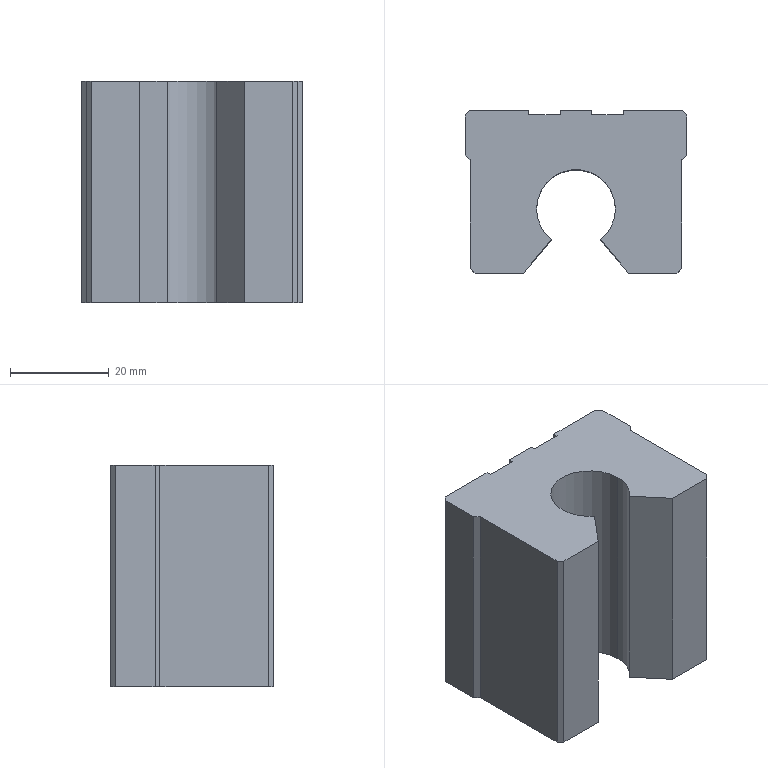Part | SolidWorks | features ICE 6, Chamfer 3, Draft 3, BaseBody 2, HoleWzd 2, Extrusion 1 | 1 solid | 52 faces | box 45 x 33 x 45 mm | volume 49974 mm3 | plane 25 | cone 16 | cylinder 11 | commonest cylinder face diameters 4.134 x8 16 x3
STEP:
#1=CARTESIAN_POINT('',(16.,44.567,212.933));
#2=VERTEX_POINT('',#1);
#3=CARTESIAN_POINT('',(16.,44.567,217.067));
#4=VERTEX_POINT('',#3);
#5=CARTESIAN_POINT('',(16.,44.567,215.));
#6=DIRECTION('',(0.,1.,0.));
#7=DIRECTION('',(0.,0.,-1.));
#8=AXIS2_PLACEMENT_3D('',#5,#6,#7);
#9=CIRCLE('',#8,2.067);
#10=EDGE_CURVE('',#2,#4,#9,.T.);
#11=ORIENTED_EDGE('',*,*,#10,.F.);
#12=CARTESIAN_POINT('',(16.,45.,212.5));
#13=VERTEX_POINT('',#12);
#14=CARTESIAN_POINT('',(16.,44.567,212.933));
#15=DIRECTION('',(0.,0.7071,-0.7071));
#16=VECTOR('',#15,1000.);
#17=LINE('',#14,#16);
#18=EDGE_CURVE('',#2,#13,#17,.T.);
#19=ORIENTED_EDGE('',*,*,#18,.T.);
#20=CARTESIAN_POINT('',(16.,45.,217.5));
#21=VERTEX_POINT('',#20);
#22=CARTESIAN_POINT('',(16.,45.,215.));
#23=DIRECTION('',(0.,-1.,0.));
#24=DIRECTION('',(0.,0.,-1.));
#25=AXIS2_PLACEMENT_3D('',#22,#23,#24);
#26=CIRCLE('',#25,2.5);
#27=EDGE_CURVE('',#21,#13,#26,.T.);
#28=ORIENTED_EDGE('',*,*,#27,.F.);
#29=CARTESIAN_POINT('',(16.,44.567,217.067));
#30=DIRECTION('',(0.,0.7071,0.7071));
#31=VECTOR('',#30,1000.);
#32=LINE('',#29,#31);
#33=EDGE_CURVE('',#4,#21,#32,.T.);
#34=ORIENTED_EDGE('',*,*,#33,.F.);
#35=EDGE_LOOP('',(#11,#19,#28,#34));
#36=FACE_OUTER_BOUND('',#35,.T.);
#37=CARTESIAN_POINT('',(16.,44.567,215.));
#38=DIRECTION('',(0.,1.,0.));
#39=DIRECTION('',(0.,0.,1.));
#40=AXIS2_PLACEMENT_3D('',#37,#38,#39);
#41=CONICAL_SURFACE('',#40,2.067,0.7854);
#42=ADVANCED_FACE('',(#36),#41,.F.);
#43=CARTESIAN_POINT('',(-16.,44.567,242.933));
#44=VERTEX_POINT('',#43);
#45=CARTESIAN_POINT('',(-16.,44.567,247.067));
#46=VERTEX_POINT('',#45);
#47=CARTESIAN_POINT('',(-16.,44.567,245.));
#48=DIRECTION('',(0.,1.,0.));
#49=DIRECTION('',(0.,0.,-1.));
#50=AXIS2_PLACEMENT_3D('',#47,#48,#49);
#51=CIRCLE('',#50,2.067);
#52=EDGE_CURVE('',#44,#46,#51,.T.);
#53=ORIENTED_EDGE('',*,*,#52,.F.);
#54=CARTESIAN_POINT('',(-16.,45.,242.5));
#55=VERTEX_POINT('',#54);
#56=CARTESIAN_POINT('',(-16.,44.567,242.933));
#57=DIRECTION('',(0.,0.7071,-0.7071));
#58=VECTOR('',#57,1000.);
#59=LINE('',#56,#58);
#60=EDGE_CURVE('',#44,#55,#59,.T.);
#61=ORIENTED_EDGE('',*,*,#60,.T.);
#62=CARTESIAN_POINT('',(-16.,45.,247.5));
#63=VERTEX_POINT('',#62);
#64=CARTESIAN_POINT('',(-16.,45.,245.));
#65=DIRECTION('',(0.,-1.,0.));
#66=DIRECTION('',(0.,0.,-1.));
#67=AXIS2_PLACEMENT_3D('',#64,#65,#66);
#68=CIRCLE('',#67,2.5);
#69=EDGE_CURVE('',#63,#55,#68,.T.);
#70=ORIENTED_EDGE('',*,*,#69,.F.);
#71=CARTESIAN_POINT('',(-16.,44.567,247.067));
#72=DIRECTION('',(0.,0.7071,0.7071));
#73=VECTOR('',#72,1000.);
#74=LINE('',#71,#73);
#75=EDGE_CURVE('',#46,#63,#74,.T.);
#76=ORIENTED_EDGE('',*,*,#75,.F.);
#77=EDGE_LOOP('',(#53,#61,#70,#76));
#78=FACE_OUTER_BOUND('',#77,.T.);
#79=CARTESIAN_POINT('',(-16.,44.567,245.));
#80=DIRECTION('',(0.,1.,0.));
#81=DIRECTION('',(0.,0.,1.));
#82=AXIS2_PLACEMENT_3D('',#79,#80,#81);
#83=CONICAL_SURFACE('',#82,2.067,0.7854);
#84=ADVANCED_FACE('',(#78),#83,.F.);
#85=CARTESIAN_POINT('',(16.,44.567,242.933));
#86=VERTEX_POINT('',#85);
#87=CARTESIAN_POINT('',(16.,44.567,247.067));
#88=VERTEX_POINT('',#87);
#89=CARTESIAN_POINT('',(16.,44.567,245.));
#90=DIRECTION('',(0.,1.,0.));
#91=DIRECTION('',(0.,0.,-1.));
#92=AXIS2_PLACEMENT_3D('',#89,#90,#91);
#93=CIRCLE('',#92,2.067);
#94=EDGE_CURVE('',#86,#88,#93,.T.);
#95=ORIENTED_EDGE('',*,*,#94,.F.);
#96=CARTESIAN_POINT('',(16.,45.,242.5));
#97=VERTEX_POINT('',#96);
#98=CARTESIAN_POINT('',(16.,44.567,242.933));
#99=DIRECTION('',(0.,0.7071,-0.7071));
#100=VECTOR('',#99,1000.);
#101=LINE('',#98,#100);
#102=EDGE_CURVE('',#86,#97,#101,.T.);
#103=ORIENTED_EDGE('',*,*,#102,.T.);
#104=CARTESIAN_POINT('',(16.,45.,247.5));
#105=VERTEX_POINT('',#104);
#106=CARTESIAN_POINT('',(16.,45.,245.));
#107=DIRECTION('',(0.,-1.,0.));
#108=DIRECTION('',(0.,0.,-1.));
#109=AXIS2_PLACEMENT_3D('',#106,#107,#108);
#110=CIRCLE('',#109,2.5);
#111=EDGE_CURVE('',#105,#97,#110,.T.);
#112=ORIENTED_EDGE('',*,*,#111,.F.);
#113=CARTESIAN_POINT('',(16.,44.567,247.067));
#114=DIRECTION('',(0.,0.7071,0.7071));
#115=VECTOR('',#114,1000.);
#116=LINE('',#113,#115);
#117=EDGE_CURVE('',#88,#105,#116,.T.);
#118=ORIENTED_EDGE('',*,*,#117,.F.);
#119=EDGE_LOOP('',(#95,#103,#112,#118));
#120=FACE_OUTER_BOUND('',#119,.T.);
#121=CARTESIAN_POINT('',(16.,44.567,245.));
#122=DIRECTION('',(0.,1.,0.));
#123=DIRECTION('',(0.,0.,1.));
#124=AXIS2_PLACEMENT_3D('',#121,#122,#123);
#125=CONICAL_SURFACE('',#124,2.067,0.7854);
#126=ADVANCED_FACE('',(#120),#125,.F.);
#127=CARTESIAN_POINT('',(-16.,44.567,212.933));
#128=VERTEX_POINT('',#127);
#129=CARTESIAN_POINT('',(-16.,44.567,217.067));
#130=VERTEX_POINT('',#129);
#131=CARTESIAN_POINT('',(-16.,44.567,215.));
#132=DIRECTION('',(0.,1.,0.));
#133=DIRECTION('',(0.,0.,-1.));
#134=AXIS2_PLACEMENT_3D('',#131,#132,#133);
#135=CIRCLE('',#134,2.067);
#136=EDGE_CURVE('',#128,#130,#135,.T.);
#137=ORIENTED_EDGE('',*,*,#136,.F.);
#138=CARTESIAN_POINT('',(-16.,45.,212.5));
#139=VERTEX_POINT('',#138);
#140=CARTESIAN_POINT('',(-16.,44.567,212.933));
#141=DIRECTION('',(0.,0.7071,-0.7071));
#142=VECTOR('',#141,1000.);
#143=LINE('',#140,#142);
#144=EDGE_CURVE('',#128,#139,#143,.T.);
#145=ORIENTED_EDGE('',*,*,#144,.T.);
#146=CARTESIAN_POINT('',(-16.,45.,217.5));
#147=VERTEX_POINT('',#146);
#148=CARTESIAN_POINT('',(-16.,45.,215.));
#149=DIRECTION('',(0.,-1.,0.));
#150=DIRECTION('',(0.,0.,-1.));
#151=AXIS2_PLACEMENT_3D('',#148,#149,#150);
#152=CIRCLE('',#151,2.5);
#153=EDGE_CURVE('',#147,#139,#152,.T.);
#154=ORIENTED_EDGE('',*,*,#153,.F.);
#155=CARTESIAN_POINT('',(-16.,44.567,217.067));
#156=DIRECTION('',(0.,0.7071,0.7071));
#157=VECTOR('',#156,1000.);
#158=LINE('',#155,#157);
#159=EDGE_CURVE('',#130,#147,#158,.T.);
#160=ORIENTED_EDGE('',*,*,#159,.F.);
#161=EDGE_LOOP('',(#137,#145,#154,#160));
#162=FACE_OUTER_BOUND('',#161,.T.);
#163=CARTESIAN_POINT('',(-16.,44.567,215.));
#164=DIRECTION('',(0.,1.,0.));
#165=DIRECTION('',(0.,0.,1.));
#166=AXIS2_PLACEMENT_3D('',#163,#164,#165);
#167=CONICAL_SURFACE('',#166,2.067,0.7854);
#168=ADVANCED_FACE('',(#162),#167,.F.);
#169=CARTESIAN_POINT('',(16.,29.393,212.933));
#170=VERTEX_POINT('',#169);
#171=CARTESIAN_POINT('',(16.,29.393,217.067));
#172=VERTEX_POINT('',#171);
#173=CARTESIAN_POINT('',(16.,29.393,215.));
#174=DIRECTION('',(0.,1.,0.));
#175=DIRECTION('',(0.,0.,1.));
#176=AXIS2_PLACEMENT_3D('',#173,#174,#175);
#177=CIRCLE('',#176,2.067);
#178=EDGE_CURVE('',#170,#172,#177,.T.);
#179=ORIENTED_EDGE('',*,*,#178,.F.);
#180=CARTESIAN_POINT('',(16.,45.,212.933));
#181=DIRECTION('',(0.,1.,0.));
#182=VECTOR('',#181,1000.);
#183=LINE('',#180,#182);
#184=EDGE_CURVE('',#170,#2,#183,.T.);
#185=ORIENTED_EDGE('',*,*,#184,.T.);
#186=ORIENTED_EDGE('',*,*,#10,.T.);
#187=CARTESIAN_POINT('',(16.,45.,217.067));
#188=DIRECTION('',(0.,1.,0.));
#189=VECTOR('',#188,1000.);
#190=LINE('',#187,#189);
#191=EDGE_CURVE('',#172,#4,#190,.T.);
#192=ORIENTED_EDGE('',*,*,#191,.F.);
#193=EDGE_LOOP('',(#179,#185,#186,#192));
#194=FACE_OUTER_BOUND('',#193,.T.);
#195=CARTESIAN_POINT('',(16.,45.,215.));
#196=DIRECTION('',(0.,1.,0.));
#197=DIRECTION('',(0.,0.,1.));
#198=AXIS2_PLACEMENT_3D('',#195,#196,#197);
#199=CYLINDRICAL_SURFACE('',#198,2.067);
#200=ADVANCED_FACE('',(#194),#199,.F.);
#201=CARTESIAN_POINT('',(16.,28.2,215.));
#202=VERTEX_POINT('',#201);
#203=CARTESIAN_POINT('',(16.,29.393,217.067));
#204=DIRECTION('',(0.,0.5,0.866));
#205=VECTOR('',#204,1000.);
#206=LINE('',#203,#205);
#207=EDGE_CURVE('',#202,#172,#206,.T.);
#208=ORIENTED_EDGE('',*,*,#207,.F.);
#209=CARTESIAN_POINT('',(16.,29.393,212.933));
#210=DIRECTION('',(0.,0.5,-0.866));
#211=VECTOR('',#210,1000.);
#212=LINE('',#209,#211);
#213=EDGE_CURVE('',#202,#170,#212,.T.);
#214=ORIENTED_EDGE('',*,*,#213,.T.);
#215=ORIENTED_EDGE('',*,*,#178,.T.);
#216=EDGE_LOOP('',(#208,#214,#215));
#217=FACE_OUTER_BOUND('',#216,.T.);
#218=CARTESIAN_POINT('',(16.,29.393,215.));
#219=DIRECTION('',(0.,1.,0.));
#220=DIRECTION('',(0.,0.,1.));
#221=AXIS2_PLACEMENT_3D('',#218,#219,#220);
#222=CONICAL_SURFACE('',#221,2.067,1.047);
#223=ADVANCED_FACE('',(#217),#222,.F.);
#224=CARTESIAN_POINT('',(16.,29.393,242.933));
#225=VERTEX_POINT('',#224);
#226=CARTESIAN_POINT('',(16.,29.393,247.067));
#227=VERTEX_POINT('',#226);
#228=CARTESIAN_POINT('',(16.,29.393,245.));
#229=DIRECTION('',(0.,1.,0.));
#230=DIRECTION('',(0.,0.,1.));
#231=AXIS2_PLACEMENT_3D('',#228,#229,#230);
#232=CIRCLE('',#231,2.067);
#233=EDGE_CURVE('',#225,#227,#232,.T.);
#234=ORIENTED_EDGE('',*,*,#233,.F.);
#235=CARTESIAN_POINT('',(16.,45.,242.933));
#236=DIRECTION('',(0.,1.,0.));
#237=VECTOR('',#236,1000.);
#238=LINE('',#235,#237);
#239=EDGE_CURVE('',#225,#86,#238,.T.);
#240=ORIENTED_EDGE('',*,*,#239,.T.);
#241=ORIENTED_EDGE('',*,*,#94,.T.);
#242=CARTESIAN_POINT('',(16.,45.,247.067));
#243=DIRECTION('',(0.,1.,0.));
#244=VECTOR('',#243,1000.);
#245=LINE('',#242,#244);
#246=EDGE_CURVE('',#227,#88,#245,.T.);
#247=ORIENTED_EDGE('',*,*,#246,.F.);
#248=EDGE_LOOP('',(#234,#240,#241,#247));
#249=FACE_OUTER_BOUND('',#248,.T.);
#250=CARTESIAN_POINT('',(16.,45.,245.));
#251=DIRECTION('',(0.,1.,0.));
#252=DIRECTION('',(0.,0.,1.));
#253=AXIS2_PLACEMENT_3D('',#250,#251,#252);
#254=CYLINDRICAL_SURFACE('',#253,2.067);
#255=ADVANCED_FACE('',(#249),#254,.F.);
#256=CARTESIAN_POINT('',(16.,28.2,245.));
#257=VERTEX_POINT('',#256);
#258=CARTESIAN_POINT('',(16.,29.393,247.067));
#259=DIRECTION('',(0.,0.5,0.866));
#260=VECTOR('',#259,1000.);
#261=LINE('',#258,#260);
#262=EDGE_CURVE('',#257,#227,#261,.T.);
#263=ORIENTED_EDGE('',*,*,#262,.F.);
#264=CARTESIAN_POINT('',(16.,29.393,242.933));
#265=DIRECTION('',(0.,0.5,-0.866));
#266=VECTOR('',#265,1000.);
#267=LINE('',#264,#266);
#268=EDGE_CURVE('',#257,#225,#267,.T.);
#269=ORIENTED_EDGE('',*,*,#268,.T.);
#270=ORIENTED_EDGE('',*,*,#233,.T.);
#271=EDGE_LOOP('',(#263,#269,#270));
#272=FACE_OUTER_BOUND('',#271,.T.);
#273=CARTESIAN_POINT('',(16.,29.393,245.));
#274=DIRECTION('',(0.,1.,0.));
#275=DIRECTION('',(0.,0.,1.));
#276=AXIS2_PLACEMENT_3D('',#273,#274,#275);
#277=CONICAL_SURFACE('',#276,2.067,1.047);
#278=ADVANCED_FACE('',(#272),#277,.F.);
#279=CARTESIAN_POINT('',(-16.,29.393,212.933));
#280=VERTEX_POINT('',#279);
#281=CARTESIAN_POINT('',(-16.,29.393,217.067));
#282=VERTEX_POINT('',#281);
#283=CARTESIAN_POINT('',(-16.,29.393,215.));
#284=DIRECTION('',(0.,1.,0.));
#285=DIRECTION('',(0.,0.,1.));
#286=AXIS2_PLACEMENT_3D('',#283,#284,#285);
#287=CIRCLE('',#286,2.067);
#288=EDGE_CURVE('',#280,#282,#287,.T.);
#289=ORIENTED_EDGE('',*,*,#288,.F.);
#290=CARTESIAN_POINT('',(-16.,45.,212.933));
#291=DIRECTION('',(0.,1.,0.));
#292=VECTOR('',#291,1000.);
#293=LINE('',#290,#292);
#294=EDGE_CURVE('',#280,#128,#293,.T.);
#295=ORIENTED_EDGE('',*,*,#294,.T.);
#296=ORIENTED_EDGE('',*,*,#136,.T.);
#297=CARTESIAN_POINT('',(-16.,45.,217.067));
#298=DIRECTION('',(0.,1.,0.));
#299=VECTOR('',#298,1000.);
#300=LINE('',#297,#299);
#301=EDGE_CURVE('',#282,#130,#300,.T.);
#302=ORIENTED_EDGE('',*,*,#301,.F.);
#303=EDGE_LOOP('',(#289,#295,#296,#302));
#304=FACE_OUTER_BOUND('',#303,.T.);
#305=CARTESIAN_POINT('',(-16.,45.,215.));
#306=DIRECTION('',(0.,1.,0.));
#307=DIRECTION('',(0.,0.,1.));
#308=AXIS2_PLACEMENT_3D('',#305,#306,#307);
#309=CYLINDRICAL_SURFACE('',#308,2.067);
#310=ADVANCED_FACE('',(#304),#309,.F.);
#311=CARTESIAN_POINT('',(-16.,28.2,215.));
#312=VERTEX_POINT('',#311);
#313=CARTESIAN_POINT('',(-16.,29.393,217.067));
#314=DIRECTION('',(0.,0.5,0.866));
#315=VECTOR('',#314,1000.);
#316=LINE('',#313,#315);
#317=EDGE_CURVE('',#312,#282,#316,.T.);
#318=ORIENTED_EDGE('',*,*,#317,.F.);
#319=CARTESIAN_POINT('',(-16.,29.393,212.933));
#320=DIRECTION('',(0.,0.5,-0.866));
#321=VECTOR('',#320,1000.);
#322=LINE('',#319,#321);
#323=EDGE_CURVE('',#312,#280,#322,.T.);
#324=ORIENTED_EDGE('',*,*,#323,.T.);
#325=ORIENTED_EDGE('',*,*,#288,.T.);
#326=EDGE_LOOP('',(#318,#324,#325));
#327=FACE_OUTER_BOUND('',#326,.T.);
#328=CARTESIAN_POINT('',(-16.,29.393,215.));
#329=DIRECTION('',(0.,1.,0.));
#330=DIRECTION('',(0.,0.,1.));
#331=AXIS2_PLACEMENT_3D('',#328,#329,#330);
#332=CONICAL_SURFACE('',#331,2.067,1.047);
#333=ADVANCED_FACE('',(#327),#332,.F.);
#334=CARTESIAN_POINT('',(-16.,29.393,242.933));
#335=VERTEX_POINT('',#334);
#336=CARTESIAN_POINT('',(-16.,29.393,247.067));
#337=VERTEX_POINT('',#336);
#338=CARTESIAN_POINT('',(-16.,29.393,245.));
#339=DIRECTION('',(0.,1.,0.));
#340=DIRECTION('',(0.,0.,1.));
#341=AXIS2_PLACEMENT_3D('',#338,#339,#340);
#342=CIRCLE('',#341,2.067);
#343=EDGE_CURVE('',#335,#337,#342,.T.);
#344=ORIENTED_EDGE('',*,*,#343,.F.);
#345=CARTESIAN_POINT('',(-16.,45.,242.933));
#346=DIRECTION('',(0.,1.,0.));
#347=VECTOR('',#346,1000.);
#348=LINE('',#345,#347);
#349=EDGE_CURVE('',#335,#44,#348,.T.);
#350=ORIENTED_EDGE('',*,*,#349,.T.);
#351=ORIENTED_EDGE('',*,*,#52,.T.);
#352=CARTESIAN_POINT('',(-16.,45.,247.067));
#353=DIRECTION('',(0.,1.,0.));
#354=VECTOR('',#353,1000.);
#355=LINE('',#352,#354);
#356=EDGE_CURVE('',#337,#46,#355,.T.);
#357=ORIENTED_EDGE('',*,*,#356,.F.);
#358=EDGE_LOOP('',(#344,#350,#351,#357));
#359=FACE_OUTER_BOUND('',#358,.T.);
#360=CARTESIAN_POINT('',(-16.,45.,245.));
#361=DIRECTION('',(0.,1.,0.));
#362=DIRECTION('',(0.,0.,1.));
#363=AXIS2_PLACEMENT_3D('',#360,#361,#362);
#364=CYLINDRICAL_SURFACE('',#363,2.067);
#365=ADVANCED_FACE('',(#359),#364,.F.);
#366=CARTESIAN_POINT('',(-16.,28.2,245.));
#367=VERTEX_POINT('',#366);
#368=CARTESIAN_POINT('',(-16.,29.393,247.067));
#369=DIRECTION('',(0.,0.5,0.866));
#370=VECTOR('',#369,1000.);
#371=LINE('',#368,#370);
#372=EDGE_CURVE('',#367,#337,#371,.T.);
#373=ORIENTED_EDGE('',*,*,#372,.F.);
#374=CARTESIAN_POINT('',(-16.,29.393,242.933));
#375=DIRECTION('',(0.,0.5,-0.866));
#376=VECTOR('',#375,1000.);
#377=LINE('',#374,#376);
#378=EDGE_CURVE('',#367,#335,#377,.T.);
#379=ORIENTED_EDGE('',*,*,#378,.T.);
#380=ORIENTED_EDGE('',*,*,#343,.T.);
#381=EDGE_LOOP('',(#373,#379,#380));
#382=FACE_OUTER_BOUND('',#381,.T.);
#383=CARTESIAN_POINT('',(-16.,29.393,245.));
#384=DIRECTION('',(0.,1.,0.));
#385=DIRECTION('',(0.,0.,1.));
#386=AXIS2_PLACEMENT_3D('',#383,#384,#385);
#387=CONICAL_SURFACE('',#386,2.067,1.047);
#388=ADVANCED_FACE('',(#382),#387,.F.);
#389=CARTESIAN_POINT('',(8.,25.,252.5));
#390=VERTEX_POINT('',#389);
#391=CARTESIAN_POINT('',(5.,18.755,252.5));
#392=VERTEX_POINT('',#391);
#393=CARTESIAN_POINT('',(0.,25.,252.5));
#394=DIRECTION('',(0.,0.,-1.));
#395=DIRECTION('',(-1.,0.,0.));
#396=AXIS2_PLACEMENT_3D('',#393,#394,#395);
#397=CIRCLE('',#396,8.);
#398=EDGE_CURVE('',#390,#392,#397,.T.);
#399=ORIENTED_EDGE('',*,*,#398,.F.);
#400=CARTESIAN_POINT('',(8.,25.,207.5));
#401=VERTEX_POINT('',#400);
#402=CARTESIAN_POINT('',(8.,25.,207.5));
#403=DIRECTION('',(0.,0.,-1.));
#404=VECTOR('',#403,1000.);
#405=LINE('',#402,#404);
#406=EDGE_CURVE('',#390,#401,#405,.T.);
#407=ORIENTED_EDGE('',*,*,#406,.T.);
#408=CARTESIAN_POINT('',(5.,18.755,207.5));
#409=VERTEX_POINT('',#408);
#410=CARTESIAN_POINT('',(0.,25.,207.5));
#411=DIRECTION('',(0.,0.,-1.));
#412=DIRECTION('',(-1.,0.,0.));
#413=AXIS2_PLACEMENT_3D('',#410,#411,#412);
#414=CIRCLE('',#413,8.);
#415=EDGE_CURVE('',#401,#409,#414,.T.);
#416=ORIENTED_EDGE('',*,*,#415,.T.);
#417=CARTESIAN_POINT('',(5.,18.755,207.5));
#418=DIRECTION('',(0.,0.,-1.));
#419=VECTOR('',#418,1000.);
#420=LINE('',#417,#419);
#421=EDGE_CURVE('',#392,#409,#420,.T.);
#422=ORIENTED_EDGE('',*,*,#421,.F.);
#423=EDGE_LOOP('',(#399,#407,#416,#422));
#424=FACE_OUTER_BOUND('',#423,.T.);
#425=CARTESIAN_POINT('',(0.,25.,207.5));
#426=DIRECTION('',(0.,0.,-1.));
#427=DIRECTION('',(-1.,0.,0.));
#428=AXIS2_PLACEMENT_3D('',#425,#426,#427);
#429=CYLINDRICAL_SURFACE('',#428,8.);
#430=ADVANCED_FACE('',(#424),#429,.F.);
#431=ORIENTED_EDGE('',*,*,#406,.F.);
#432=CARTESIAN_POINT('',(-8.,25.,252.5));
#433=VERTEX_POINT('',#432);
#434=CARTESIAN_POINT('',(0.,25.,252.5));
#435=DIRECTION('',(0.,0.,-1.));
#436=DIRECTION('',(-1.,0.,0.));
#437=AXIS2_PLACEMENT_3D('',#434,#435,#436);
#438=CIRCLE('',#437,8.);
#439=EDGE_CURVE('',#433,#390,#438,.T.);
#440=ORIENTED_EDGE('',*,*,#439,.F.);
#441=CARTESIAN_POINT('',(-8.,25.,207.5));
#442=VERTEX_POINT('',#441);
#443=CARTESIAN_POINT('',(-8.,25.,207.5));
#444=DIRECTION('',(0.,0.,-1.));
#445=VECTOR('',#444,1000.);
#446=LINE('',#443,#445);
#447=EDGE_CURVE('',#433,#442,#446,.T.);
#448=ORIENTED_EDGE('',*,*,#447,.T.);
#449=CARTESIAN_POINT('',(0.,25.,207.5));
#450=DIRECTION('',(0.,0.,-1.));
#451=DIRECTION('',(-1.,0.,0.));
#452=AXIS2_PLACEMENT_3D('',#449,#450,#451);
#453=CIRCLE('',#452,8.);
#454=EDGE_CURVE('',#442,#401,#453,.T.);
#455=ORIENTED_EDGE('',*,*,#454,.T.);
#456=EDGE_LOOP('',(#431,#440,#448,#455));
#457=FACE_OUTER_BOUND('',#456,.T.);
#458=CARTESIAN_POINT('',(0.,25.,207.5));
#459=DIRECTION('',(0.,0.,-1.));
#460=DIRECTION('',(-1.,0.,0.));
#461=AXIS2_PLACEMENT_3D('',#458,#459,#460);
#462=CYLINDRICAL_SURFACE('',#461,8.);
#463=ADVANCED_FACE('',(#457),#462,.F.);
#464=CARTESIAN_POINT('',(-9.6,45.,252.5));
#465=VERTEX_POINT('',#464);
#466=CARTESIAN_POINT('',(-21.6,45.,252.5));
#467=VERTEX_POINT('',#466);
#468=CARTESIAN_POINT('',(22.5,45.,252.5));
#469=DIRECTION('',(-1.,0.,0.));
#470=VECTOR('',#469,1000.);
#471=LINE('',#468,#470);
#472=EDGE_CURVE('',#465,#467,#471,.T.);
#473=ORIENTED_EDGE('',*,*,#472,.T.);
#474=CARTESIAN_POINT('',(-22.5,44.1,252.5));
#475=VERTEX_POINT('',#474);
#476=CARTESIAN_POINT('',(0.45,67.05,252.5));
#477=DIRECTION('',(-0.7071,-0.7071,0.));
#478=VECTOR('',#477,1000.);
#479=LINE('',#476,#478);
#480=EDGE_CURVE('',#467,#475,#479,.T.);
#481=ORIENTED_EDGE('',*,*,#480,.T.);
#482=CARTESIAN_POINT('',(-22.5,36.,252.5));
#483=VERTEX_POINT('',#482);
#484=CARTESIAN_POINT('',(-22.5,45.,252.5));
#485=DIRECTION('',(0.,-1.,0.));
#486=VECTOR('',#485,1000.);
#487=LINE('',#484,#486);
#488=EDGE_CURVE('',#475,#483,#487,.T.);
#489=ORIENTED_EDGE('',*,*,#488,.T.);
#490=CARTESIAN_POINT('',(-21.5,35.,252.5));
#491=VERTEX_POINT('',#490);
#492=CARTESIAN_POINT('',(-4.5,18.,252.5));
#493=DIRECTION('',(-0.7071,0.7071,0.));
#494=VECTOR('',#493,1000.);
#495=LINE('',#492,#494);
#496=EDGE_CURVE('',#491,#483,#495,.T.);
#497=ORIENTED_EDGE('',*,*,#496,.F.);
#498=CARTESIAN_POINT('',(-21.5,13.,252.5));
#499=VERTEX_POINT('',#498);
#500=CARTESIAN_POINT('',(-21.5,12.,252.5));
#501=DIRECTION('',(0.,1.,0.));
#502=VECTOR('',#501,1000.);
#503=LINE('',#500,#502);
#504=EDGE_CURVE('',#499,#491,#503,.T.);
#505=ORIENTED_EDGE('',*,*,#504,.F.);
#506=CARTESIAN_POINT('',(-20.5,12.,252.5));
#507=VERTEX_POINT('',#506);
#508=CARTESIAN_POINT('',(-15.5,7.,252.5));
#509=DIRECTION('',(0.7071,-0.7071,0.));
#510=VECTOR('',#509,1000.);
#511=LINE('',#508,#510);
#512=EDGE_CURVE('',#499,#507,#511,.T.);
#513=ORIENTED_EDGE('',*,*,#512,.T.);
#514=CARTESIAN_POINT('',(-10.668,12.,252.5));
#515=VERTEX_POINT('',#514);
#516=CARTESIAN_POINT('',(22.5,12.,252.5));
#517=DIRECTION('',(-1.,0.,0.));
#518=VECTOR('',#517,1000.);
#519=LINE('',#516,#518);
#520=EDGE_CURVE('',#515,#507,#519,.T.);
#521=ORIENTED_EDGE('',*,*,#520,.F.);
#522=CARTESIAN_POINT('',(-5.,18.755,252.5));
#523=VERTEX_POINT('',#522);
#524=CARTESIAN_POINT('',(19.285,47.697,252.5));
#525=DIRECTION('',(-0.6428,-0.766,0.));
#526=VECTOR('',#525,1000.);
#527=LINE('',#524,#526);
#528=EDGE_CURVE('',#523,#515,#527,.T.);
#529=ORIENTED_EDGE('',*,*,#528,.F.);
#530=CARTESIAN_POINT('',(0.,25.,252.5));
#531=DIRECTION('',(0.,0.,-1.));
#532=DIRECTION('',(-1.,0.,0.));
#533=AXIS2_PLACEMENT_3D('',#530,#531,#532);
#534=CIRCLE('',#533,8.);
#535=EDGE_CURVE('',#523,#433,#534,.T.);
#536=ORIENTED_EDGE('',*,*,#535,.T.);
#537=ORIENTED_EDGE('',*,*,#439,.T.);
#538=ORIENTED_EDGE('',*,*,#398,.T.);
#539=CARTESIAN_POINT('',(10.668,12.,252.5));
#540=VERTEX_POINT('',#539);
#541=CARTESIAN_POINT('',(10.668,12.,252.5));
#542=CARTESIAN_POINT('',(8.779,14.252,252.5));
#543=CARTESIAN_POINT('',(6.889,16.503,252.5));
#544=CARTESIAN_POINT('',(5.,18.755,252.5));
#545=B_SPLINE_CURVE_WITH_KNOTS('',3,(#541,#542,#543,#544),.UNSPECIFIED.,.F.,.F.,(4,4),(0.,1.),.UNSPECIFIED.);
#546=EDGE_CURVE('',#540,#392,#545,.T.);
#547=ORIENTED_EDGE('',*,*,#546,.F.);
#548=CARTESIAN_POINT('',(20.5,12.,252.5));
#549=VERTEX_POINT('',#548);
#550=CARTESIAN_POINT('',(22.5,12.,252.5));
#551=DIRECTION('',(-1.,0.,0.));
#552=VECTOR('',#551,1000.);
#553=LINE('',#550,#552);
#554=EDGE_CURVE('',#549,#540,#553,.T.);
#555=ORIENTED_EDGE('',*,*,#554,.F.);
#556=CARTESIAN_POINT('',(21.5,13.,252.5));
#557=VERTEX_POINT('',#556);
#558=CARTESIAN_POINT('',(38.,29.5,252.5));
#559=DIRECTION('',(0.7071,0.7071,0.));
#560=VECTOR('',#559,1000.);
#561=LINE('',#558,#560);
#562=EDGE_CURVE('',#549,#557,#561,.T.);
#563=ORIENTED_EDGE('',*,*,#562,.T.);
#564=CARTESIAN_POINT('',(21.5,35.,252.5));
#565=VERTEX_POINT('',#564);
#566=CARTESIAN_POINT('',(21.5,36.,252.5));
#567=DIRECTION('',(0.,-1.,0.));
#568=VECTOR('',#567,1000.);
#569=LINE('',#566,#568);
#570=EDGE_CURVE('',#565,#557,#569,.T.);
#571=ORIENTED_EDGE('',*,*,#570,.F.);
#572=CARTESIAN_POINT('',(22.5,36.,252.5));
#573=VERTEX_POINT('',#572);
#574=CARTESIAN_POINT('',(27.,40.5,252.5));
#575=DIRECTION('',(-0.7071,-0.7071,0.));
#576=VECTOR('',#575,1000.);
#577=LINE('',#574,#576);
#578=EDGE_CURVE('',#573,#565,#577,.T.);
#579=ORIENTED_EDGE('',*,*,#578,.F.);
#580=CARTESIAN_POINT('',(22.5,44.1,252.5));
#581=VERTEX_POINT('',#580);
#582=CARTESIAN_POINT('',(22.5,45.,252.5));
#583=DIRECTION('',(0.,-1.,0.));
#584=VECTOR('',#583,1000.);
#585=LINE('',#582,#584);
#586=EDGE_CURVE('',#581,#573,#585,.T.);
#587=ORIENTED_EDGE('',*,*,#586,.F.);
#588=CARTESIAN_POINT('',(21.6,45.,252.5));
#589=VERTEX_POINT('',#588);
#590=CARTESIAN_POINT('',(22.05,44.55,252.5));
#591=DIRECTION('',(-0.7071,0.7071,0.));
#592=VECTOR('',#591,1000.);
#593=LINE('',#590,#592);
#594=EDGE_CURVE('',#581,#589,#593,.T.);
#595=ORIENTED_EDGE('',*,*,#594,.T.);
#596=CARTESIAN_POINT('',(9.6,45.,252.5));
#597=VERTEX_POINT('',#596);
#598=CARTESIAN_POINT('',(22.5,45.,252.5));
#599=DIRECTION('',(-1.,0.,0.));
#600=VECTOR('',#599,1000.);
#601=LINE('',#598,#600);
#602=EDGE_CURVE('',#589,#597,#601,.T.);
#603=ORIENTED_EDGE('',*,*,#602,.T.);
#604=CARTESIAN_POINT('',(9.6,44.1,252.5));
#605=VERTEX_POINT('',#604);
#606=CARTESIAN_POINT('',(9.6,44.1,252.5));
#607=DIRECTION('',(0.,1.,0.));
#608=VECTOR('',#607,1000.);
#609=LINE('',#606,#608);
#610=EDGE_CURVE('',#605,#597,#609,.T.);
#611=ORIENTED_EDGE('',*,*,#610,.F.);
#612=CARTESIAN_POINT('',(3.2,44.1,252.5));
#613=VERTEX_POINT('',#612);
#614=CARTESIAN_POINT('',(3.2,44.1,252.5));
#615=DIRECTION('',(1.,0.,0.));
#616=VECTOR('',#615,1000.);
#617=LINE('',#614,#616);
#618=EDGE_CURVE('',#613,#605,#617,.T.);
#619=ORIENTED_EDGE('',*,*,#618,.F.);
#620=CARTESIAN_POINT('',(3.2,45.,252.5));
#621=VERTEX_POINT('',#620);
#622=CARTESIAN_POINT('',(3.2,45.,252.5));
#623=DIRECTION('',(0.,-1.,0.));
#624=VECTOR('',#623,1000.);
#625=LINE('',#622,#624);
#626=EDGE_CURVE('',#621,#613,#625,.T.);
#627=ORIENTED_EDGE('',*,*,#626,.F.);
#628=CARTESIAN_POINT('',(-3.2,45.,252.5));
#629=VERTEX_POINT('',#628);
#630=CARTESIAN_POINT('',(22.5,45.,252.5));
#631=DIRECTION('',(-1.,0.,0.));
#632=VECTOR('',#631,1000.);
#633=LINE('',#630,#632);
#634=EDGE_CURVE('',#621,#629,#633,.T.);
#635=ORIENTED_EDGE('',*,*,#634,.T.);
#636=CARTESIAN_POINT('',(-3.2,44.1,252.5));
#637=VERTEX_POINT('',#636);
#638=CARTESIAN_POINT('',(-3.2,44.1,252.5));
#639=DIRECTION('',(0.,1.,0.));
#640=VECTOR('',#639,1000.);
#641=LINE('',#638,#640);
#642=EDGE_CURVE('',#637,#629,#641,.T.);
#643=ORIENTED_EDGE('',*,*,#642,.F.);
#644=CARTESIAN_POINT('',(-9.6,44.1,252.5));
#645=VERTEX_POINT('',#644);
#646=CARTESIAN_POINT('',(-9.6,44.1,252.5));
#647=DIRECTION('',(1.,0.,0.));
#648=VECTOR('',#647,1000.);
#649=LINE('',#646,#648);
#650=EDGE_CURVE('',#645,#637,#649,.T.);
#651=ORIENTED_EDGE('',*,*,#650,.F.);
#652=CARTESIAN_POINT('',(-9.6,45.,252.5));
#653=DIRECTION('',(0.,-1.,0.));
#654=VECTOR('',#653,1000.);
#655=LINE('',#652,#654);
#656=EDGE_CURVE('',#465,#645,#655,.T.);
#657=ORIENTED_EDGE('',*,*,#656,.F.);
#658=EDGE_LOOP('',(#473,#481,#489,#497,#505,#513,#521,#529,#536,#537,#538,#547,#555,#563,#571,#579,#587,#595,#603,#611,#619,#627,#635,#643,#651,#657));
#659=FACE_OUTER_BOUND('',#658,.T.);
#660=CARTESIAN_POINT('',(22.5,45.,252.5));
#661=DIRECTION('',(0.,0.,1.));
#662=DIRECTION('',(1.,0.,0.));
#663=AXIS2_PLACEMENT_3D('',#660,#661,#662);
#664=PLANE('',#663);
#665=ADVANCED_FACE('',(#659),#664,.T.);
#666=ORIENTED_EDGE('',*,*,#520,.T.);
#667=CARTESIAN_POINT('',(-20.5,12.,207.5));
#668=VERTEX_POINT('',#667);
#669=CARTESIAN_POINT('',(-20.5,12.,207.5));
#670=DIRECTION('',(0.,0.,-1.));
#671=VECTOR('',#670,1000.);
#672=LINE('',#669,#671);
#673=EDGE_CURVE('',#507,#668,#672,.T.);
#674=ORIENTED_EDGE('',*,*,#673,.T.);
#675=CARTESIAN_POINT('',(-10.668,12.,207.5));
#676=VERTEX_POINT('',#675);
#677=CARTESIAN_POINT('',(-22.5,12.,207.5));
#678=DIRECTION('',(1.,0.,0.));
#679=VECTOR('',#678,1000.);
#680=LINE('',#677,#679);
#681=EDGE_CURVE('',#668,#676,#680,.T.);
#682=ORIENTED_EDGE('',*,*,#681,.T.);
#683=CARTESIAN_POINT('',(-10.668,12.,207.5));
#684=DIRECTION('',(0.,0.,1.));
#685=VECTOR('',#684,1000.);
#686=LINE('',#683,#685);
#687=EDGE_CURVE('',#676,#515,#686,.T.);
#688=ORIENTED_EDGE('',*,*,#687,.T.);
#689=EDGE_LOOP('',(#666,#674,#682,#688));
#690=FACE_OUTER_BOUND('',#689,.T.);
#691=CARTESIAN_POINT('',(0.,12.,0.));
#692=DIRECTION('',(0.,-1.,0.));
#693=DIRECTION('',(0.,0.,-1.));
#694=AXIS2_PLACEMENT_3D('',#691,#692,#693);
#695=PLANE('',#694);
#696=ADVANCED_FACE('',(#690),#695,.T.);
#697=ORIENTED_EDGE('',*,*,#111,.T.);
#698=CARTESIAN_POINT('',(16.,45.,245.));
#699=DIRECTION('',(0.,-1.,0.));
#700=DIRECTION('',(0.,0.,-1.));
#701=AXIS2_PLACEMENT_3D('',#698,#699,#700);
#702=CIRCLE('',#701,2.5);
#703=EDGE_CURVE('',#97,#105,#702,.T.);
#704=ORIENTED_EDGE('',*,*,#703,.T.);
#705=EDGE_LOOP('',(#697,#704));
#706=FACE_BOUND('',#705,.T.);
#707=ORIENTED_EDGE('',*,*,#27,.T.);
#708=CARTESIAN_POINT('',(16.,45.,215.));
#709=DIRECTION('',(0.,-1.,0.));
#710=DIRECTION('',(0.,0.,-1.));
#711=AXIS2_PLACEMENT_3D('',#708,#709,#710);
#712=CIRCLE('',#711,2.5);
#713=EDGE_CURVE('',#13,#21,#712,.T.);
#714=ORIENTED_EDGE('',*,*,#713,.T.);
#715=EDGE_LOOP('',(#707,#714));
#716=FACE_BOUND('',#715,.T.);
#717=ORIENTED_EDGE('',*,*,#602,.F.);
#718=CARTESIAN_POINT('',(21.6,45.,207.5));
#719=VERTEX_POINT('',#718);
#720=CARTESIAN_POINT('',(21.6,45.,207.5));
#721=DIRECTION('',(0.,0.,-1.));
#722=VECTOR('',#721,1000.);
#723=LINE('',#720,#722);
#724=EDGE_CURVE('',#589,#719,#723,.T.);
#725=ORIENTED_EDGE('',*,*,#724,.T.);
#726=CARTESIAN_POINT('',(9.6,45.,207.5));
#727=VERTEX_POINT('',#726);
#728=CARTESIAN_POINT('',(-22.5,45.,207.5));
#729=DIRECTION('',(1.,0.,0.));
#730=VECTOR('',#729,1000.);
#731=LINE('',#728,#730);
#732=EDGE_CURVE('',#727,#719,#731,.T.);
#733=ORIENTED_EDGE('',*,*,#732,.F.);
#734=CARTESIAN_POINT('',(9.6,45.,207.5));
#735=DIRECTION('',(0.,0.,1.));
#736=VECTOR('',#735,1000.);
#737=LINE('',#734,#736);
#738=EDGE_CURVE('',#727,#597,#737,.T.);
#739=ORIENTED_EDGE('',*,*,#738,.T.);
#740=EDGE_LOOP('',(#717,#725,#733,#739));
#741=FACE_OUTER_BOUND('',#740,.T.);
#742=CARTESIAN_POINT('',(0.,45.,0.));
#743=DIRECTION('',(0.,-1.,0.));
#744=DIRECTION('',(0.,0.,-1.));
#745=AXIS2_PLACEMENT_3D('',#742,#743,#744);
#746=PLANE('',#745);
#747=ADVANCED_FACE('',(#706,#716,#741),#746,.F.);
#748=ORIENTED_EDGE('',*,*,#634,.F.);
#749=CARTESIAN_POINT('',(3.2,45.,207.5));
#750=VERTEX_POINT('',#749);
#751=CARTESIAN_POINT('',(3.2,45.,207.5));
#752=DIRECTION('',(0.,0.,1.));
#753=VECTOR('',#752,1000.);
#754=LINE('',#751,#753);
#755=EDGE_CURVE('',#750,#621,#754,.T.);
#756=ORIENTED_EDGE('',*,*,#755,.F.);
#757=CARTESIAN_POINT('',(-3.2,45.,207.5));
#758=VERTEX_POINT('',#757);
#759=CARTESIAN_POINT('',(-22.5,45.,207.5));
#760=DIRECTION('',(1.,0.,0.));
#761=VECTOR('',#760,1000.);
#762=LINE('',#759,#761);
#763=EDGE_CURVE('',#758,#750,#762,.T.);
#764=ORIENTED_EDGE('',*,*,#763,.F.);
#765=CARTESIAN_POINT('',(-3.2,45.,207.5));
#766=DIRECTION('',(0.,0.,1.));
#767=VECTOR('',#766,1000.);
#768=LINE('',#765,#767);
#769=EDGE_CURVE('',#758,#629,#768,.T.);
#770=ORIENTED_EDGE('',*,*,#769,.T.);
#771=EDGE_LOOP('',(#748,#756,#764,#770));
#772=FACE_OUTER_BOUND('',#771,.T.);
#773=CARTESIAN_POINT('',(0.,45.,0.));
#774=DIRECTION('',(0.,-1.,0.));
#775=DIRECTION('',(0.,0.,-1.));
#776=AXIS2_PLACEMENT_3D('',#773,#774,#775);
#777=PLANE('',#776);
#778=ADVANCED_FACE('',(#772),#777,.F.);
#779=CARTESIAN_POINT('',(22.5,44.1,207.5));
#780=VERTEX_POINT('',#779);
#781=CARTESIAN_POINT('',(22.5,36.,207.5));
#782=VERTEX_POINT('',#781);
#783=CARTESIAN_POINT('',(22.5,45.,207.5));
#784=DIRECTION('',(0.,-1.,0.));
#785=VECTOR('',#784,1000.);
#786=LINE('',#783,#785);
#787=EDGE_CURVE('',#780,#782,#786,.T.);
#788=ORIENTED_EDGE('',*,*,#787,.F.);
#789=CARTESIAN_POINT('',(22.5,44.1,252.5));
#790=DIRECTION('',(0.,0.,1.));
#791=VECTOR('',#790,1000.);
#792=LINE('',#789,#791);
#793=EDGE_CURVE('',#780,#581,#792,.T.);
#794=ORIENTED_EDGE('',*,*,#793,.T.);
#795=ORIENTED_EDGE('',*,*,#586,.T.);
#796=CARTESIAN_POINT('',(22.5,36.,207.5));
#797=DIRECTION('',(0.,0.,1.));
#798=VECTOR('',#797,1000.);
#799=LINE('',#796,#798);
#800=EDGE_CURVE('',#782,#573,#799,.T.);
#801=ORIENTED_EDGE('',*,*,#800,.F.);
#802=EDGE_LOOP('',(#788,#794,#795,#801));
#803=FACE_OUTER_BOUND('',#802,.T.);
#804=CARTESIAN_POINT('',(22.5,45.,207.5));
#805=DIRECTION('',(1.,0.,0.));
#806=DIRECTION('',(0.,0.,-1.));
#807=AXIS2_PLACEMENT_3D('',#804,#805,#806);
#808=PLANE('',#807);
#809=ADVANCED_FACE('',(#803),#808,.T.);
#810=CARTESIAN_POINT('',(-22.5,44.1,207.5));
#811=VERTEX_POINT('',#810);
#812=CARTESIAN_POINT('',(-22.5,36.,207.5));
#813=VERTEX_POINT('',#812);
#814=CARTESIAN_POINT('',(-22.5,45.,207.5));
#815=DIRECTION('',(0.,-1.,0.));
#816=VECTOR('',#815,1000.);
#817=LINE('',#814,#816);
#818=EDGE_CURVE('',#811,#813,#817,.T.);
#819=ORIENTED_EDGE('',*,*,#818,.F.);
#820=CARTESIAN_POINT('',(-21.6,45.,207.5));
#821=VERTEX_POINT('',#820);
#822=CARTESIAN_POINT('',(-22.05,44.55,207.5));
#823=DIRECTION('',(0.7071,0.7071,0.));
#824=VECTOR('',#823,1000.);
#825=LINE('',#822,#824);
#826=EDGE_CURVE('',#811,#821,#825,.T.);
#827=ORIENTED_EDGE('',*,*,#826,.T.);
#828=CARTESIAN_POINT('',(-9.6,45.,207.5));
#829=VERTEX_POINT('',#828);
#830=CARTESIAN_POINT('',(-22.5,45.,207.5));
#831=DIRECTION('',(1.,0.,0.));
#832=VECTOR('',#831,1000.);
#833=LINE('',#830,#832);
#834=EDGE_CURVE('',#821,#829,#833,.T.);
#835=ORIENTED_EDGE('',*,*,#834,.T.);
#836=CARTESIAN_POINT('',(-9.6,44.1,207.5));
#837=VERTEX_POINT('',#836);
#838=CARTESIAN_POINT('',(-9.6,45.,207.5));
#839=DIRECTION('',(0.,-1.,0.));
#840=VECTOR('',#839,1000.);
#841=LINE('',#838,#840);
#842=EDGE_CURVE('',#829,#837,#841,.T.);
#843=ORIENTED_EDGE('',*,*,#842,.T.);
#844=CARTESIAN_POINT('',(-3.2,44.1,207.5));
#845=VERTEX_POINT('',#844);
#846=CARTESIAN_POINT('',(-9.6,44.1,207.5));
#847=DIRECTION('',(1.,0.,0.));
#848=VECTOR('',#847,1000.);
#849=LINE('',#846,#848);
#850=EDGE_CURVE('',#837,#845,#849,.T.);
#851=ORIENTED_EDGE('',*,*,#850,.T.);
#852=CARTESIAN_POINT('',(-3.2,44.1,207.5));
#853=DIRECTION('',(0.,1.,0.));
#854=VECTOR('',#853,1000.);
#855=LINE('',#852,#854);
#856=EDGE_CURVE('',#845,#758,#855,.T.);
#857=ORIENTED_EDGE('',*,*,#856,.T.);
#858=ORIENTED_EDGE('',*,*,#763,.T.);
#859=CARTESIAN_POINT('',(3.2,44.1,207.5));
#860=VERTEX_POINT('',#859);
#861=CARTESIAN_POINT('',(3.2,45.,207.5));
#862=DIRECTION('',(0.,-1.,0.));
#863=VECTOR('',#862,1000.);
#864=LINE('',#861,#863);
#865=EDGE_CURVE('',#750,#860,#864,.T.);
#866=ORIENTED_EDGE('',*,*,#865,.T.);
#867=CARTESIAN_POINT('',(9.6,44.1,207.5));
#868=VERTEX_POINT('',#867);
#869=CARTESIAN_POINT('',(3.2,44.1,207.5));
#870=DIRECTION('',(1.,0.,0.));
#871=VECTOR('',#870,1000.);
#872=LINE('',#869,#871);
#873=EDGE_CURVE('',#860,#868,#872,.T.);
#874=ORIENTED_EDGE('',*,*,#873,.T.);
#875=CARTESIAN_POINT('',(9.6,44.1,207.5));
#876=DIRECTION('',(0.,1.,0.));
#877=VECTOR('',#876,1000.);
#878=LINE('',#875,#877);
#879=EDGE_CURVE('',#868,#727,#878,.T.);
#880=ORIENTED_EDGE('',*,*,#879,.T.);
#881=ORIENTED_EDGE('',*,*,#732,.T.);
#882=CARTESIAN_POINT('',(-0.45,67.05,207.5));
#883=DIRECTION('',(0.7071,-0.7071,0.));
#884=VECTOR('',#883,1000.);
#885=LINE('',#882,#884);
#886=EDGE_CURVE('',#719,#780,#885,.T.);
#887=ORIENTED_EDGE('',*,*,#886,.T.);
#888=ORIENTED_EDGE('',*,*,#787,.T.);
#889=CARTESIAN_POINT('',(21.5,35.,207.5));
#890=VERTEX_POINT('',#889);
#891=CARTESIAN_POINT('',(22.5,36.,207.5));
#892=DIRECTION('',(-0.7071,-0.7071,0.));
#893=VECTOR('',#892,1000.);
#894=LINE('',#891,#893);
#895=EDGE_CURVE('',#782,#890,#894,.T.);
#896=ORIENTED_EDGE('',*,*,#895,.T.);
#897=CARTESIAN_POINT('',(21.5,13.,207.5));
#898=VERTEX_POINT('',#897);
#899=CARTESIAN_POINT('',(21.5,36.,207.5));
#900=DIRECTION('',(0.,-1.,0.));
#901=VECTOR('',#900,1000.);
#902=LINE('',#899,#901);
#903=EDGE_CURVE('',#890,#898,#902,.T.);
#904=ORIENTED_EDGE('',*,*,#903,.T.);
#905=CARTESIAN_POINT('',(20.5,12.,207.5));
#906=VERTEX_POINT('',#905);
#907=CARTESIAN_POINT('',(15.5,7.,207.5));
#908=DIRECTION('',(-0.7071,-0.7071,0.));
#909=VECTOR('',#908,1000.);
#910=LINE('',#907,#909);
#911=EDGE_CURVE('',#898,#906,#910,.T.);
#912=ORIENTED_EDGE('',*,*,#911,.T.);
#913=CARTESIAN_POINT('',(10.668,12.,207.5));
#914=VERTEX_POINT('',#913);
#915=CARTESIAN_POINT('',(-22.5,12.,207.5));
#916=DIRECTION('',(1.,0.,0.));
#917=VECTOR('',#916,1000.);
#918=LINE('',#915,#917);
#919=EDGE_CURVE('',#914,#906,#918,.T.);
#920=ORIENTED_EDGE('',*,*,#919,.F.);
#921=CARTESIAN_POINT('',(10.668,12.,207.5));
#922=CARTESIAN_POINT('',(8.779,14.252,207.5));
#923=CARTESIAN_POINT('',(6.889,16.503,207.5));
#924=CARTESIAN_POINT('',(5.,18.755,207.5));
#925=B_SPLINE_CURVE_WITH_KNOTS('',3,(#921,#922,#923,#924),.UNSPECIFIED.,.F.,.F.,(4,4),(0.,1.),.UNSPECIFIED.);
#926=EDGE_CURVE('',#914,#409,#925,.T.);
#927=ORIENTED_EDGE('',*,*,#926,.T.);
#928=ORIENTED_EDGE('',*,*,#415,.F.);
#929=ORIENTED_EDGE('',*,*,#454,.F.);
#930=CARTESIAN_POINT('',(-5.,18.755,207.5));
#931=VERTEX_POINT('',#930);
#932=CARTESIAN_POINT('',(0.,25.,207.5));
#933=DIRECTION('',(0.,0.,-1.));
#934=DIRECTION('',(-1.,0.,0.));
#935=AXIS2_PLACEMENT_3D('',#932,#933,#934);
#936=CIRCLE('',#935,8.);
#937=EDGE_CURVE('',#931,#442,#936,.T.);
#938=ORIENTED_EDGE('',*,*,#937,.F.);
#939=CARTESIAN_POINT('',(-10.668,12.,207.5));
#940=DIRECTION('',(-0.6428,-0.766,0.));
#941=VECTOR('',#940,1000.);
#942=LINE('',#939,#941);
#943=EDGE_CURVE('',#931,#676,#942,.T.);
#944=ORIENTED_EDGE('',*,*,#943,.T.);
#945=ORIENTED_EDGE('',*,*,#681,.F.);
#946=CARTESIAN_POINT('',(-21.5,13.,207.5));
#947=VERTEX_POINT('',#946);
#948=CARTESIAN_POINT('',(-38.,29.5,207.5));
#949=DIRECTION('',(-0.7071,0.7071,0.));
#950=VECTOR('',#949,1000.);
#951=LINE('',#948,#950);
#952=EDGE_CURVE('',#668,#947,#951,.T.);
#953=ORIENTED_EDGE('',*,*,#952,.T.);
#954=CARTESIAN_POINT('',(-21.5,35.,207.5));
#955=VERTEX_POINT('',#954);
#956=CARTESIAN_POINT('',(-21.5,12.,207.5));
#957=DIRECTION('',(0.,1.,0.));
#958=VECTOR('',#957,1000.);
#959=LINE('',#956,#958);
#960=EDGE_CURVE('',#947,#955,#959,.T.);
#961=ORIENTED_EDGE('',*,*,#960,.T.);
#962=CARTESIAN_POINT('',(-22.5,36.,207.5));
#963=DIRECTION('',(-0.7071,0.7071,0.));
#964=VECTOR('',#963,1000.);
#965=LINE('',#962,#964);
#966=EDGE_CURVE('',#955,#813,#965,.T.);
#967=ORIENTED_EDGE('',*,*,#966,.T.);
#968=EDGE_LOOP('',(#819,#827,#835,#843,#851,#857,#858,#866,#874,#880,#881,#887,#888,#896,#904,#912,#920,#927,#928,#929,#938,#944,#945,#953,#961,#967));
#969=FACE_OUTER_BOUND('',#968,.T.);
#970=CARTESIAN_POINT('',(-22.5,45.,207.5));
#971=DIRECTION('',(0.,0.,-1.));
#972=DIRECTION('',(-1.,0.,0.));
#973=AXIS2_PLACEMENT_3D('',#970,#971,#972);
#974=PLANE('',#973);
#975=ADVANCED_FACE('',(#969),#974,.T.);
#976=ORIENTED_EDGE('',*,*,#488,.F.);
#977=CARTESIAN_POINT('',(-22.5,44.1,207.5));
#978=DIRECTION('',(0.,0.,-1.));
#979=VECTOR('',#978,1000.);
#980=LINE('',#977,#979);
#981=EDGE_CURVE('',#475,#811,#980,.T.);
#982=ORIENTED_EDGE('',*,*,#981,.T.);
#983=ORIENTED_EDGE('',*,*,#818,.T.);
#984=CARTESIAN_POINT('',(-22.5,36.,207.5));
#985=DIRECTION('',(0.,0.,1.));
#986=VECTOR('',#985,1000.);
#987=LINE('',#984,#986);
#988=EDGE_CURVE('',#813,#483,#987,.T.);
#989=ORIENTED_EDGE('',*,*,#988,.T.);
#990=EDGE_LOOP('',(#976,#982,#983,#989));
#991=FACE_OUTER_BOUND('',#990,.T.);
#992=CARTESIAN_POINT('',(-22.5,45.,252.5));
#993=DIRECTION('',(-1.,0.,0.));
#994=DIRECTION('',(0.,0.,1.));
#995=AXIS2_PLACEMENT_3D('',#992,#993,#994);
#996=PLANE('',#995);
#997=ADVANCED_FACE('',(#991),#996,.T.);
#998=ORIENTED_EDGE('',*,*,#153,.T.);
#999=CARTESIAN_POINT('',(-16.,45.,215.));
#1000=DIRECTION('',(0.,-1.,0.));
#1001=DIRECTION('',(0.,0.,-1.));
#1002=AXIS2_PLACEMENT_3D('',#999,#1000,#1001);
#1003=CIRCLE('',#1002,2.5);
#1004=EDGE_CURVE('',#139,#147,#1003,.T.);
#1005=ORIENTED_EDGE('',*,*,#1004,.T.);
#1006=EDGE_LOOP('',(#998,#1005));
#1007=FACE_BOUND('',#1006,.T.);
#1008=ORIENTED_EDGE('',*,*,#69,.T.);
#1009=CARTESIAN_POINT('',(-16.,45.,245.));
#1010=DIRECTION('',(0.,-1.,0.));
#1011=DIRECTION('',(0.,0.,-1.));
#1012=AXIS2_PLACEMENT_3D('',#1009,#1010,#1011);
#1013=CIRCLE('',#1012,2.5);
#1014=EDGE_CURVE('',#55,#63,#1013,.T.);
#1015=ORIENTED_EDGE('',*,*,#1014,.T.);
#1016=EDGE_LOOP('',(#1008,#1015));
#1017=FACE_BOUND('',#1016,.T.);
#1018=ORIENTED_EDGE('',*,*,#834,.F.);
#1019=CARTESIAN_POINT('',(-21.6,45.,252.5));
#1020=DIRECTION('',(0.,0.,1.));
#1021=VECTOR('',#1020,1000.);
#1022=LINE('',#1019,#1021);
#1023=EDGE_CURVE('',#821,#467,#1022,.T.);
#1024=ORIENTED_EDGE('',*,*,#1023,.T.);
#1025=ORIENTED_EDGE('',*,*,#472,.F.);
#1026=CARTESIAN_POINT('',(-9.6,45.,207.5));
#1027=DIRECTION('',(0.,0.,1.));
#1028=VECTOR('',#1027,1000.);
#1029=LINE('',#1026,#1028);
#1030=EDGE_CURVE('',#829,#465,#1029,.T.);
#1031=ORIENTED_EDGE('',*,*,#1030,.F.);
#1032=EDGE_LOOP('',(#1018,#1024,#1025,#1031));
#1033=FACE_OUTER_BOUND('',#1032,.T.);
#1034=CARTESIAN_POINT('',(0.,45.,0.));
#1035=DIRECTION('',(0.,-1.,0.));
#1036=DIRECTION('',(0.,0.,-1.));
#1037=AXIS2_PLACEMENT_3D('',#1034,#1035,#1036);
#1038=PLANE('',#1037);
#1039=ADVANCED_FACE('',(#1007,#1017,#1033),#1038,.F.);
#1040=ORIENTED_EDGE('',*,*,#919,.T.);
#1041=CARTESIAN_POINT('',(20.5,12.,252.5));
#1042=DIRECTION('',(0.,0.,1.));
#1043=VECTOR('',#1042,1000.);
#1044=LINE('',#1041,#1043);
#1045=EDGE_CURVE('',#906,#549,#1044,.T.);
#1046=ORIENTED_EDGE('',*,*,#1045,.T.);
#1047=ORIENTED_EDGE('',*,*,#554,.T.);
#1048=CARTESIAN_POINT('',(10.668,12.,207.5));
#1049=DIRECTION('',(0.,0.,1.));
#1050=VECTOR('',#1049,1000.);
#1051=LINE('',#1048,#1050);
#1052=EDGE_CURVE('',#914,#540,#1051,.T.);
#1053=ORIENTED_EDGE('',*,*,#1052,.F.);
#1054=EDGE_LOOP('',(#1040,#1046,#1047,#1053));
#1055=FACE_OUTER_BOUND('',#1054,.T.);
#1056=CARTESIAN_POINT('',(0.,12.,0.));
#1057=DIRECTION('',(0.,-1.,0.));
#1058=DIRECTION('',(0.,0.,-1.));
#1059=AXIS2_PLACEMENT_3D('',#1056,#1057,#1058);
#1060=PLANE('',#1059);
#1061=ADVANCED_FACE('',(#1055),#1060,.T.);
#1062=ORIENTED_EDGE('',*,*,#642,.T.);
#1063=ORIENTED_EDGE('',*,*,#769,.F.);
#1064=ORIENTED_EDGE('',*,*,#856,.F.);
#1065=CARTESIAN_POINT('',(-3.2,44.1,207.5));
#1066=DIRECTION('',(0.,0.,1.));
#1067=VECTOR('',#1066,1000.);
#1068=LINE('',#1065,#1067);
#1069=EDGE_CURVE('',#845,#637,#1068,.T.);
#1070=ORIENTED_EDGE('',*,*,#1069,.T.);
#1071=EDGE_LOOP('',(#1062,#1063,#1064,#1070));
#1072=FACE_OUTER_BOUND('',#1071,.T.);
#1073=CARTESIAN_POINT('',(-3.2,44.1,207.5));
#1074=DIRECTION('',(1.,0.,0.));
#1075=DIRECTION('',(0.,0.,-1.));
#1076=AXIS2_PLACEMENT_3D('',#1073,#1074,#1075);
#1077=PLANE('',#1076);
#1078=ADVANCED_FACE('',(#1072),#1077,.F.);
#1079=ORIENTED_EDGE('',*,*,#650,.T.);
#1080=ORIENTED_EDGE('',*,*,#1069,.F.);
#1081=ORIENTED_EDGE('',*,*,#850,.F.);
#1082=CARTESIAN_POINT('',(-9.6,44.1,207.5));
#1083=DIRECTION('',(0.,0.,1.));
#1084=VECTOR('',#1083,1000.);
#1085=LINE('',#1082,#1084);
#1086=EDGE_CURVE('',#837,#645,#1085,.T.);
#1087=ORIENTED_EDGE('',*,*,#1086,.T.);
#1088=EDGE_LOOP('',(#1079,#1080,#1081,#1087));
#1089=FACE_OUTER_BOUND('',#1088,.T.);
#1090=CARTESIAN_POINT('',(-9.6,44.1,207.5));
#1091=DIRECTION('',(0.,-1.,0.));
#1092=DIRECTION('',(0.,0.,-1.));
#1093=AXIS2_PLACEMENT_3D('',#1090,#1091,#1092);
#1094=PLANE('',#1093);
#1095=ADVANCED_FACE('',(#1089),#1094,.F.);
#1096=ORIENTED_EDGE('',*,*,#656,.T.);
#1097=ORIENTED_EDGE('',*,*,#1086,.F.);
#1098=ORIENTED_EDGE('',*,*,#842,.F.);
#1099=ORIENTED_EDGE('',*,*,#1030,.T.);
#1100=EDGE_LOOP('',(#1096,#1097,#1098,#1099));
#1101=FACE_OUTER_BOUND('',#1100,.T.);
#1102=CARTESIAN_POINT('',(-9.6,45.,207.5));
#1103=DIRECTION('',(-1.,0.,0.));
#1104=DIRECTION('',(0.,0.,1.));
#1105=AXIS2_PLACEMENT_3D('',#1102,#1103,#1104);
#1106=PLANE('',#1105);
#1107=ADVANCED_FACE('',(#1101),#1106,.F.);
#1108=ORIENTED_EDGE('',*,*,#610,.T.);
#1109=ORIENTED_EDGE('',*,*,#738,.F.);
#1110=ORIENTED_EDGE('',*,*,#879,.F.);
#1111=CARTESIAN_POINT('',(9.6,44.1,207.5));
#1112=DIRECTION('',(0.,0.,1.));
#1113=VECTOR('',#1112,1000.);
#1114=LINE('',#1111,#1113);
#1115=EDGE_CURVE('',#868,#605,#1114,.T.);
#1116=ORIENTED_EDGE('',*,*,#1115,.T.);
#1117=EDGE_LOOP('',(#1108,#1109,#1110,#1116));
#1118=FACE_OUTER_BOUND('',#1117,.T.);
#1119=CARTESIAN_POINT('',(9.6,44.1,207.5));
#1120=DIRECTION('',(1.,0.,0.));
#1121=DIRECTION('',(0.,1.,0.));
#1122=AXIS2_PLACEMENT_3D('',#1119,#1120,#1121);
#1123=PLANE('',#1122);
#1124=ADVANCED_FACE('',(#1118),#1123,.F.);
#1125=ORIENTED_EDGE('',*,*,#618,.T.);
#1126=ORIENTED_EDGE('',*,*,#1115,.F.);
#1127=ORIENTED_EDGE('',*,*,#873,.F.);
#1128=CARTESIAN_POINT('',(3.2,44.1,207.5));
#1129=DIRECTION('',(0.,0.,1.));
#1130=VECTOR('',#1129,1000.);
#1131=LINE('',#1128,#1130);
#1132=EDGE_CURVE('',#860,#613,#1131,.T.);
#1133=ORIENTED_EDGE('',*,*,#1132,.T.);
#1134=EDGE_LOOP('',(#1125,#1126,#1127,#1133));
#1135=FACE_OUTER_BOUND('',#1134,.T.);
#1136=CARTESIAN_POINT('',(3.2,44.1,207.5));
#1137=DIRECTION('',(0.,-1.,0.));
#1138=DIRECTION('',(0.,0.,-1.));
#1139=AXIS2_PLACEMENT_3D('',#1136,#1137,#1138);
#1140=PLANE('',#1139);
#1141=ADVANCED_FACE('',(#1135),#1140,.F.);
#1142=ORIENTED_EDGE('',*,*,#626,.T.);
#1143=ORIENTED_EDGE('',*,*,#1132,.F.);
#1144=ORIENTED_EDGE('',*,*,#865,.F.);
#1145=ORIENTED_EDGE('',*,*,#755,.T.);
#1146=EDGE_LOOP('',(#1142,#1143,#1144,#1145));
#1147=FACE_OUTER_BOUND('',#1146,.T.);
#1148=CARTESIAN_POINT('',(3.2,45.,207.5));
#1149=DIRECTION('',(-1.,0.,0.));
#1150=DIRECTION('',(0.,0.,1.));
#1151=AXIS2_PLACEMENT_3D('',#1148,#1149,#1150);
#1152=PLANE('',#1151);
#1153=ADVANCED_FACE('',(#1147),#1152,.F.);
#1154=ORIENTED_EDGE('',*,*,#570,.T.);
#1155=CARTESIAN_POINT('',(21.5,13.,207.5));
#1156=DIRECTION('',(0.,0.,-1.));
#1157=VECTOR('',#1156,1000.);
#1158=LINE('',#1155,#1157);
#1159=EDGE_CURVE('',#557,#898,#1158,.T.);
#1160=ORIENTED_EDGE('',*,*,#1159,.T.);
#1161=ORIENTED_EDGE('',*,*,#903,.F.);
#1162=CARTESIAN_POINT('',(21.5,35.,207.5));
#1163=DIRECTION('',(0.,0.,1.));
#1164=VECTOR('',#1163,1000.);
#1165=LINE('',#1162,#1164);
#1166=EDGE_CURVE('',#890,#565,#1165,.T.);
#1167=ORIENTED_EDGE('',*,*,#1166,.T.);
#1168=EDGE_LOOP('',(#1154,#1160,#1161,#1167));
#1169=FACE_OUTER_BOUND('',#1168,.T.);
#1170=CARTESIAN_POINT('',(21.5,36.,207.5));
#1171=DIRECTION('',(-1.,0.,0.));
#1172=DIRECTION('',(0.,-1.,0.));
#1173=AXIS2_PLACEMENT_3D('',#1170,#1171,#1172);
#1174=PLANE('',#1173);
#1175=ADVANCED_FACE('',(#1169),#1174,.F.);
#1176=ORIENTED_EDGE('',*,*,#578,.T.);
#1177=ORIENTED_EDGE('',*,*,#1166,.F.);
#1178=ORIENTED_EDGE('',*,*,#895,.F.);
#1179=ORIENTED_EDGE('',*,*,#800,.T.);
#1180=EDGE_LOOP('',(#1176,#1177,#1178,#1179));
#1181=FACE_OUTER_BOUND('',#1180,.T.);
#1182=CARTESIAN_POINT('',(22.5,36.,207.5));
#1183=DIRECTION('',(0.7071,-0.7071,0.));
#1184=DIRECTION('',(0.7071,0.7071,0.));
#1185=AXIS2_PLACEMENT_3D('',#1182,#1183,#1184);
#1186=PLANE('',#1185);
#1187=ADVANCED_FACE('',(#1181),#1186,.T.);
#1188=ORIENTED_EDGE('',*,*,#943,.F.);
#1189=CARTESIAN_POINT('',(-5.,18.755,207.5));
#1190=DIRECTION('',(0.,0.,1.));
#1191=VECTOR('',#1190,1000.);
#1192=LINE('',#1189,#1191);
#1193=EDGE_CURVE('',#931,#523,#1192,.T.);
#1194=ORIENTED_EDGE('',*,*,#1193,.T.);
#1195=ORIENTED_EDGE('',*,*,#528,.T.);
#1196=ORIENTED_EDGE('',*,*,#687,.F.);
#1197=EDGE_LOOP('',(#1188,#1194,#1195,#1196));
#1198=FACE_OUTER_BOUND('',#1197,.T.);
#1199=CARTESIAN_POINT('',(-10.668,12.,207.5));
#1200=DIRECTION('',(0.766,-0.6428,0.));
#1201=DIRECTION('',(0.6428,0.766,0.));
#1202=AXIS2_PLACEMENT_3D('',#1199,#1200,#1201);
#1203=PLANE('',#1202);
#1204=ADVANCED_FACE('',(#1198),#1203,.T.);
#1205=ORIENTED_EDGE('',*,*,#546,.T.);
#1206=ORIENTED_EDGE('',*,*,#421,.T.);
#1207=ORIENTED_EDGE('',*,*,#926,.F.);
#1208=ORIENTED_EDGE('',*,*,#1052,.T.);
#1209=EDGE_LOOP('',(#1205,#1206,#1207,#1208));
#1210=FACE_OUTER_BOUND('',#1209,.T.);
#1211=CARTESIAN_POINT('',(5.,18.755,207.5));
#1212=DIRECTION('',(0.766,0.6428,0.));
#1213=DIRECTION('',(-0.6428,0.766,0.));
#1214=AXIS2_PLACEMENT_3D('',#1211,#1212,#1213);
#1215=PLANE('',#1214);
#1216=ADVANCED_FACE('',(#1210),#1215,.F.);
#1217=ORIENTED_EDGE('',*,*,#960,.F.);
#1218=CARTESIAN_POINT('',(-21.5,13.,252.5));
#1219=DIRECTION('',(0.,0.,1.));
#1220=VECTOR('',#1219,1000.);
#1221=LINE('',#1218,#1220);
#1222=EDGE_CURVE('',#947,#499,#1221,.T.);
#1223=ORIENTED_EDGE('',*,*,#1222,.T.);
#1224=ORIENTED_EDGE('',*,*,#504,.T.);
#1225=CARTESIAN_POINT('',(-21.5,35.,207.5));
#1226=DIRECTION('',(0.,0.,1.));
#1227=VECTOR('',#1226,1000.);
#1228=LINE('',#1225,#1227);
#1229=EDGE_CURVE('',#955,#491,#1228,.T.);
#1230=ORIENTED_EDGE('',*,*,#1229,.F.);
#1231=EDGE_LOOP('',(#1217,#1223,#1224,#1230));
#1232=FACE_OUTER_BOUND('',#1231,.T.);
#1233=CARTESIAN_POINT('',(-21.5,12.,207.5));
#1234=DIRECTION('',(1.,0.,0.));
#1235=DIRECTION('',(0.,0.,-1.));
#1236=AXIS2_PLACEMENT_3D('',#1233,#1234,#1235);
#1237=PLANE('',#1236);
#1238=ADVANCED_FACE('',(#1232),#1237,.F.);
#1239=ORIENTED_EDGE('',*,*,#496,.T.);
#1240=ORIENTED_EDGE('',*,*,#988,.F.);
#1241=ORIENTED_EDGE('',*,*,#966,.F.);
#1242=ORIENTED_EDGE('',*,*,#1229,.T.);
#1243=EDGE_LOOP('',(#1239,#1240,#1241,#1242));
#1244=FACE_OUTER_BOUND('',#1243,.T.);
#1245=CARTESIAN_POINT('',(-22.5,36.,207.5));
#1246=DIRECTION('',(-0.7071,-0.7071,0.));
#1247=DIRECTION('',(0.7071,-0.7071,0.));
#1248=AXIS2_PLACEMENT_3D('',#1245,#1246,#1247);
#1249=PLANE('',#1248);
#1250=ADVANCED_FACE('',(#1244),#1249,.T.);
#1251=ORIENTED_EDGE('',*,*,#447,.F.);
#1252=ORIENTED_EDGE('',*,*,#535,.F.);
#1253=ORIENTED_EDGE('',*,*,#1193,.F.);
#1254=ORIENTED_EDGE('',*,*,#937,.T.);
#1255=EDGE_LOOP('',(#1251,#1252,#1253,#1254));
#1256=FACE_OUTER_BOUND('',#1255,.T.);
#1257=CARTESIAN_POINT('',(0.,25.,207.5));
#1258=DIRECTION('',(0.,0.,-1.));
#1259=DIRECTION('',(-1.,0.,0.));
#1260=AXIS2_PLACEMENT_3D('',#1257,#1258,#1259);
#1261=CYLINDRICAL_SURFACE('',#1260,8.);
#1262=ADVANCED_FACE('',(#1256),#1261,.F.);
#1263=ORIENTED_EDGE('',*,*,#378,.F.);
#1264=ORIENTED_EDGE('',*,*,#372,.T.);
#1265=CARTESIAN_POINT('',(-16.,29.393,245.));
#1266=DIRECTION('',(0.,1.,0.));
#1267=DIRECTION('',(0.,0.,1.));
#1268=AXIS2_PLACEMENT_3D('',#1265,#1266,#1267);
#1269=CIRCLE('',#1268,2.067);
#1270=EDGE_CURVE('',#337,#335,#1269,.T.);
#1271=ORIENTED_EDGE('',*,*,#1270,.T.);
#1272=EDGE_LOOP('',(#1263,#1264,#1271));
#1273=FACE_OUTER_BOUND('',#1272,.T.);
#1274=CARTESIAN_POINT('',(-16.,29.393,245.));
#1275=DIRECTION('',(0.,1.,0.));
#1276=DIRECTION('',(0.,0.,1.));
#1277=AXIS2_PLACEMENT_3D('',#1274,#1275,#1276);
#1278=CONICAL_SURFACE('',#1277,2.067,1.047);
#1279=ADVANCED_FACE('',(#1273),#1278,.F.);
#1280=ORIENTED_EDGE('',*,*,#349,.F.);
#1281=ORIENTED_EDGE('',*,*,#1270,.F.);
#1282=ORIENTED_EDGE('',*,*,#356,.T.);
#1283=CARTESIAN_POINT('',(-16.,44.567,245.));
#1284=DIRECTION('',(0.,1.,0.));
#1285=DIRECTION('',(0.,0.,-1.));
#1286=AXIS2_PLACEMENT_3D('',#1283,#1284,#1285);
#1287=CIRCLE('',#1286,2.067);
#1288=EDGE_CURVE('',#46,#44,#1287,.T.);
#1289=ORIENTED_EDGE('',*,*,#1288,.T.);
#1290=EDGE_LOOP('',(#1280,#1281,#1282,#1289));
#1291=FACE_OUTER_BOUND('',#1290,.T.);
#1292=CARTESIAN_POINT('',(-16.,45.,245.));
#1293=DIRECTION('',(0.,1.,0.));
#1294=DIRECTION('',(0.,0.,1.));
#1295=AXIS2_PLACEMENT_3D('',#1292,#1293,#1294);
#1296=CYLINDRICAL_SURFACE('',#1295,2.067);
#1297=ADVANCED_FACE('',(#1291),#1296,.F.);
#1298=ORIENTED_EDGE('',*,*,#323,.F.);
#1299=ORIENTED_EDGE('',*,*,#317,.T.);
#1300=CARTESIAN_POINT('',(-16.,29.393,215.));
#1301=DIRECTION('',(0.,1.,0.));
#1302=DIRECTION('',(0.,0.,1.));
#1303=AXIS2_PLACEMENT_3D('',#1300,#1301,#1302);
#1304=CIRCLE('',#1303,2.067);
#1305=EDGE_CURVE('',#282,#280,#1304,.T.);
#1306=ORIENTED_EDGE('',*,*,#1305,.T.);
#1307=EDGE_LOOP('',(#1298,#1299,#1306));
#1308=FACE_OUTER_BOUND('',#1307,.T.);
#1309=CARTESIAN_POINT('',(-16.,29.393,215.));
#1310=DIRECTION('',(0.,1.,0.));
#1311=DIRECTION('',(0.,0.,1.));
#1312=AXIS2_PLACEMENT_3D('',#1309,#1310,#1311);
#1313=CONICAL_SURFACE('',#1312,2.067,1.047);
#1314=ADVANCED_FACE('',(#1308),#1313,.F.);
#1315=ORIENTED_EDGE('',*,*,#294,.F.);
#1316=ORIENTED_EDGE('',*,*,#1305,.F.);
#1317=ORIENTED_EDGE('',*,*,#301,.T.);
#1318=CARTESIAN_POINT('',(-16.,44.567,215.));
#1319=DIRECTION('',(0.,1.,0.));
#1320=DIRECTION('',(0.,0.,-1.));
#1321=AXIS2_PLACEMENT_3D('',#1318,#1319,#1320);
#1322=CIRCLE('',#1321,2.067);
#1323=EDGE_CURVE('',#130,#128,#1322,.T.);
#1324=ORIENTED_EDGE('',*,*,#1323,.T.);
#1325=EDGE_LOOP('',(#1315,#1316,#1317,#1324));
#1326=FACE_OUTER_BOUND('',#1325,.T.);
#1327=CARTESIAN_POINT('',(-16.,45.,215.));
#1328=DIRECTION('',(0.,1.,0.));
#1329=DIRECTION('',(0.,0.,1.));
#1330=AXIS2_PLACEMENT_3D('',#1327,#1328,#1329);
#1331=CYLINDRICAL_SURFACE('',#1330,2.067);
#1332=ADVANCED_FACE('',(#1326),#1331,.F.);
#1333=ORIENTED_EDGE('',*,*,#268,.F.);
#1334=ORIENTED_EDGE('',*,*,#262,.T.);
#1335=CARTESIAN_POINT('',(16.,29.393,245.));
#1336=DIRECTION('',(0.,1.,0.));
#1337=DIRECTION('',(0.,0.,1.));
#1338=AXIS2_PLACEMENT_3D('',#1335,#1336,#1337);
#1339=CIRCLE('',#1338,2.067);
#1340=EDGE_CURVE('',#227,#225,#1339,.T.);
#1341=ORIENTED_EDGE('',*,*,#1340,.T.);
#1342=EDGE_LOOP('',(#1333,#1334,#1341));
#1343=FACE_OUTER_BOUND('',#1342,.T.);
#1344=CARTESIAN_POINT('',(16.,29.393,245.));
#1345=DIRECTION('',(0.,1.,0.));
#1346=DIRECTION('',(0.,0.,1.));
#1347=AXIS2_PLACEMENT_3D('',#1344,#1345,#1346);
#1348=CONICAL_SURFACE('',#1347,2.067,1.047);
#1349=ADVANCED_FACE('',(#1343),#1348,.F.);
#1350=ORIENTED_EDGE('',*,*,#239,.F.);
#1351=ORIENTED_EDGE('',*,*,#1340,.F.);
#1352=ORIENTED_EDGE('',*,*,#246,.T.);
#1353=CARTESIAN_POINT('',(16.,44.567,245.));
#1354=DIRECTION('',(0.,1.,0.));
#1355=DIRECTION('',(0.,0.,-1.));
#1356=AXIS2_PLACEMENT_3D('',#1353,#1354,#1355);
#1357=CIRCLE('',#1356,2.067);
#1358=EDGE_CURVE('',#88,#86,#1357,.T.);
#1359=ORIENTED_EDGE('',*,*,#1358,.T.);
#1360=EDGE_LOOP('',(#1350,#1351,#1352,#1359));
#1361=FACE_OUTER_BOUND('',#1360,.T.);
#1362=CARTESIAN_POINT('',(16.,45.,245.));
#1363=DIRECTION('',(0.,1.,0.));
#1364=DIRECTION('',(0.,0.,1.));
#1365=AXIS2_PLACEMENT_3D('',#1362,#1363,#1364);
#1366=CYLINDRICAL_SURFACE('',#1365,2.067);
#1367=ADVANCED_FACE('',(#1361),#1366,.F.);
#1368=ORIENTED_EDGE('',*,*,#213,.F.);
#1369=ORIENTED_EDGE('',*,*,#207,.T.);
#1370=CARTESIAN_POINT('',(16.,29.393,215.));
#1371=DIRECTION('',(0.,1.,0.));
#1372=DIRECTION('',(0.,0.,1.));
#1373=AXIS2_PLACEMENT_3D('',#1370,#1371,#1372);
#1374=CIRCLE('',#1373,2.067);
#1375=EDGE_CURVE('',#172,#170,#1374,.T.);
#1376=ORIENTED_EDGE('',*,*,#1375,.T.);
#1377=EDGE_LOOP('',(#1368,#1369,#1376));
#1378=FACE_OUTER_BOUND('',#1377,.T.);
#1379=CARTESIAN_POINT('',(16.,29.393,215.));
#1380=DIRECTION('',(0.,1.,0.));
#1381=DIRECTION('',(0.,0.,1.));
#1382=AXIS2_PLACEMENT_3D('',#1379,#1380,#1381);
#1383=CONICAL_SURFACE('',#1382,2.067,1.047);
#1384=ADVANCED_FACE('',(#1378),#1383,.F.);
#1385=ORIENTED_EDGE('',*,*,#184,.F.);
#1386=ORIENTED_EDGE('',*,*,#1375,.F.);
#1387=ORIENTED_EDGE('',*,*,#191,.T.);
#1388=CARTESIAN_POINT('',(16.,44.567,215.));
#1389=DIRECTION('',(0.,1.,0.));
#1390=DIRECTION('',(0.,0.,-1.));
#1391=AXIS2_PLACEMENT_3D('',#1388,#1389,#1390);
#1392=CIRCLE('',#1391,2.067);
#1393=EDGE_CURVE('',#4,#2,#1392,.T.);
#1394=ORIENTED_EDGE('',*,*,#1393,.T.);
#1395=EDGE_LOOP('',(#1385,#1386,#1387,#1394));
#1396=FACE_OUTER_BOUND('',#1395,.T.);
#1397=CARTESIAN_POINT('',(16.,45.,215.));
#1398=DIRECTION('',(0.,1.,0.));
#1399=DIRECTION('',(0.,0.,1.));
#1400=AXIS2_PLACEMENT_3D('',#1397,#1398,#1399);
#1401=CYLINDRICAL_SURFACE('',#1400,2.067);
#1402=ADVANCED_FACE('',(#1396),#1401,.F.);
#1403=ORIENTED_EDGE('',*,*,#144,.F.);
#1404=ORIENTED_EDGE('',*,*,#1323,.F.);
#1405=ORIENTED_EDGE('',*,*,#159,.T.);
#1406=ORIENTED_EDGE('',*,*,#1004,.F.);
#1407=EDGE_LOOP('',(#1403,#1404,#1405,#1406));
#1408=FACE_OUTER_BOUND('',#1407,.T.);
#1409=CARTESIAN_POINT('',(-16.,44.567,215.));
#1410=DIRECTION('',(0.,1.,0.));
#1411=DIRECTION('',(0.,0.,1.));
#1412=AXIS2_PLACEMENT_3D('',#1409,#1410,#1411);
#1413=CONICAL_SURFACE('',#1412,2.067,0.7854);
#1414=ADVANCED_FACE('',(#1408),#1413,.F.);
#1415=ORIENTED_EDGE('',*,*,#102,.F.);
#1416=ORIENTED_EDGE('',*,*,#1358,.F.);
#1417=ORIENTED_EDGE('',*,*,#117,.T.);
#1418=ORIENTED_EDGE('',*,*,#703,.F.);
#1419=EDGE_LOOP('',(#1415,#1416,#1417,#1418));
#1420=FACE_OUTER_BOUND('',#1419,.T.);
#1421=CARTESIAN_POINT('',(16.,44.567,245.));
#1422=DIRECTION('',(0.,1.,0.));
#1423=DIRECTION('',(0.,0.,1.));
#1424=AXIS2_PLACEMENT_3D('',#1421,#1422,#1423);
#1425=CONICAL_SURFACE('',#1424,2.067,0.7854);
#1426=ADVANCED_FACE('',(#1420),#1425,.F.);
#1427=ORIENTED_EDGE('',*,*,#60,.F.);
#1428=ORIENTED_EDGE('',*,*,#1288,.F.);
#1429=ORIENTED_EDGE('',*,*,#75,.T.);
#1430=ORIENTED_EDGE('',*,*,#1014,.F.);
#1431=EDGE_LOOP('',(#1427,#1428,#1429,#1430));
#1432=FACE_OUTER_BOUND('',#1431,.T.);
#1433=CARTESIAN_POINT('',(-16.,44.567,245.));
#1434=DIRECTION('',(0.,1.,0.));
#1435=DIRECTION('',(0.,0.,1.));
#1436=AXIS2_PLACEMENT_3D('',#1433,#1434,#1435);
#1437=CONICAL_SURFACE('',#1436,2.067,0.7854);
#1438=ADVANCED_FACE('',(#1432),#1437,.F.);
#1439=ORIENTED_EDGE('',*,*,#18,.F.);
#1440=ORIENTED_EDGE('',*,*,#1393,.F.);
#1441=ORIENTED_EDGE('',*,*,#33,.T.);
#1442=ORIENTED_EDGE('',*,*,#713,.F.);
#1443=EDGE_LOOP('',(#1439,#1440,#1441,#1442));
#1444=FACE_OUTER_BOUND('',#1443,.T.);
#1445=CARTESIAN_POINT('',(16.,44.567,215.));
#1446=DIRECTION('',(0.,1.,0.));
#1447=DIRECTION('',(0.,0.,1.));
#1448=AXIS2_PLACEMENT_3D('',#1445,#1446,#1447);
#1449=CONICAL_SURFACE('',#1448,2.067,0.7854);
#1450=ADVANCED_FACE('',(#1444),#1449,.F.);
#1451=ORIENTED_EDGE('',*,*,#911,.F.);
#1452=ORIENTED_EDGE('',*,*,#1159,.F.);
#1453=ORIENTED_EDGE('',*,*,#562,.F.);
#1454=ORIENTED_EDGE('',*,*,#1045,.F.);
#1455=EDGE_LOOP('',(#1451,#1452,#1453,#1454));
#1456=FACE_OUTER_BOUND('',#1455,.T.);
#1457=CARTESIAN_POINT('',(20.5,12.,0.));
#1458=DIRECTION('',(0.7071,-0.7071,0.));
#1459=DIRECTION('',(0.,0.,-1.));
#1460=AXIS2_PLACEMENT_3D('',#1457,#1458,#1459);
#1461=PLANE('',#1460);
#1462=ADVANCED_FACE('',(#1456),#1461,.T.);
#1463=ORIENTED_EDGE('',*,*,#952,.F.);
#1464=ORIENTED_EDGE('',*,*,#673,.F.);
#1465=ORIENTED_EDGE('',*,*,#512,.F.);
#1466=ORIENTED_EDGE('',*,*,#1222,.F.);
#1467=EDGE_LOOP('',(#1463,#1464,#1465,#1466));
#1468=FACE_OUTER_BOUND('',#1467,.T.);
#1469=CARTESIAN_POINT('',(-21.5,13.,207.5));
#1470=DIRECTION('',(-0.7071,-0.7071,0.));
#1471=DIRECTION('',(0.,0.,-1.));
#1472=AXIS2_PLACEMENT_3D('',#1469,#1470,#1471);
#1473=PLANE('',#1472);
#1474=ADVANCED_FACE('',(#1468),#1473,.T.);
#1475=ORIENTED_EDGE('',*,*,#480,.F.);
#1476=ORIENTED_EDGE('',*,*,#1023,.F.);
#1477=ORIENTED_EDGE('',*,*,#826,.F.);
#1478=ORIENTED_EDGE('',*,*,#981,.F.);
#1479=EDGE_LOOP('',(#1475,#1476,#1477,#1478));
#1480=FACE_OUTER_BOUND('',#1479,.T.);
#1481=CARTESIAN_POINT('',(-22.5,44.1,252.5));
#1482=DIRECTION('',(-0.7071,0.7071,0.));
#1483=DIRECTION('',(0.,0.,1.));
#1484=AXIS2_PLACEMENT_3D('',#1481,#1482,#1483);
#1485=PLANE('',#1484);
#1486=ADVANCED_FACE('',(#1480),#1485,.T.);
#1487=ORIENTED_EDGE('',*,*,#886,.F.);
#1488=ORIENTED_EDGE('',*,*,#724,.F.);
#1489=ORIENTED_EDGE('',*,*,#594,.F.);
#1490=ORIENTED_EDGE('',*,*,#793,.F.);
#1491=EDGE_LOOP('',(#1487,#1488,#1489,#1490));
#1492=FACE_OUTER_BOUND('',#1491,.T.);
#1493=CARTESIAN_POINT('',(22.5,44.1,207.5));
#1494=DIRECTION('',(0.7071,0.7071,0.));
#1495=DIRECTION('',(0.,0.,-1.));
#1496=AXIS2_PLACEMENT_3D('',#1493,#1494,#1495);
#1497=PLANE('',#1496);
#1498=ADVANCED_FACE('',(#1492),#1497,.T.);
#1499=CLOSED_SHELL('',(#42,#84,#126,#168,#200,#223,#255,#278,#310,#333,#365,#388,#430,#463,#665,#696,#747,#778,#809,#975,#997,#1039,#1061,#1078,#1095,#1107,#1124,#1141,#1153,#1175,#1187,#1204,#1216,#1238,#1250,#1262,#1279,#1297,#1314,#1332,#1349,#1367,#1384,#1402,#1414,#1426,#1438,#1450,#1462,#1474,#1486,#1498));
#1500=MANIFOLD_SOLID_BREP('',#1499);
#1501=CARTESIAN_POINT('',(0.,0.,0.));
#1502=DIRECTION('',(0.,0.,1.));
#1503=DIRECTION('',(1.,0.,0.));
#1504=AXIS2_PLACEMENT_3D('',#1501,#1502,#1503);
#1505=(LENGTH_UNIT()NAMED_UNIT(*)SI_UNIT(.MILLI.,.METRE.));
#1506=UNCERTAINTY_MEASURE_WITH_UNIT(LENGTH_MEASURE(0.00001),#1505,'','');
#1507=(NAMED_UNIT(*)PLANE_ANGLE_UNIT()SI_UNIT($,.RADIAN.));
#1508=(NAMED_UNIT(*)SI_UNIT($,.STERADIAN.)SOLID_ANGLE_UNIT());
#1509=(GEOMETRIC_REPRESENTATION_CONTEXT(3)GLOBAL_UNCERTAINTY_ASSIGNED_CONTEXT((#1506))GLOBAL_UNIT_ASSIGNED_CONTEXT((#1505,#1507,#1508))REPRESENTATION_CONTEXT('',''));
#1510=ADVANCED_BREP_SHAPE_REPRESENTATION('',(#1500,#1504),#1509);